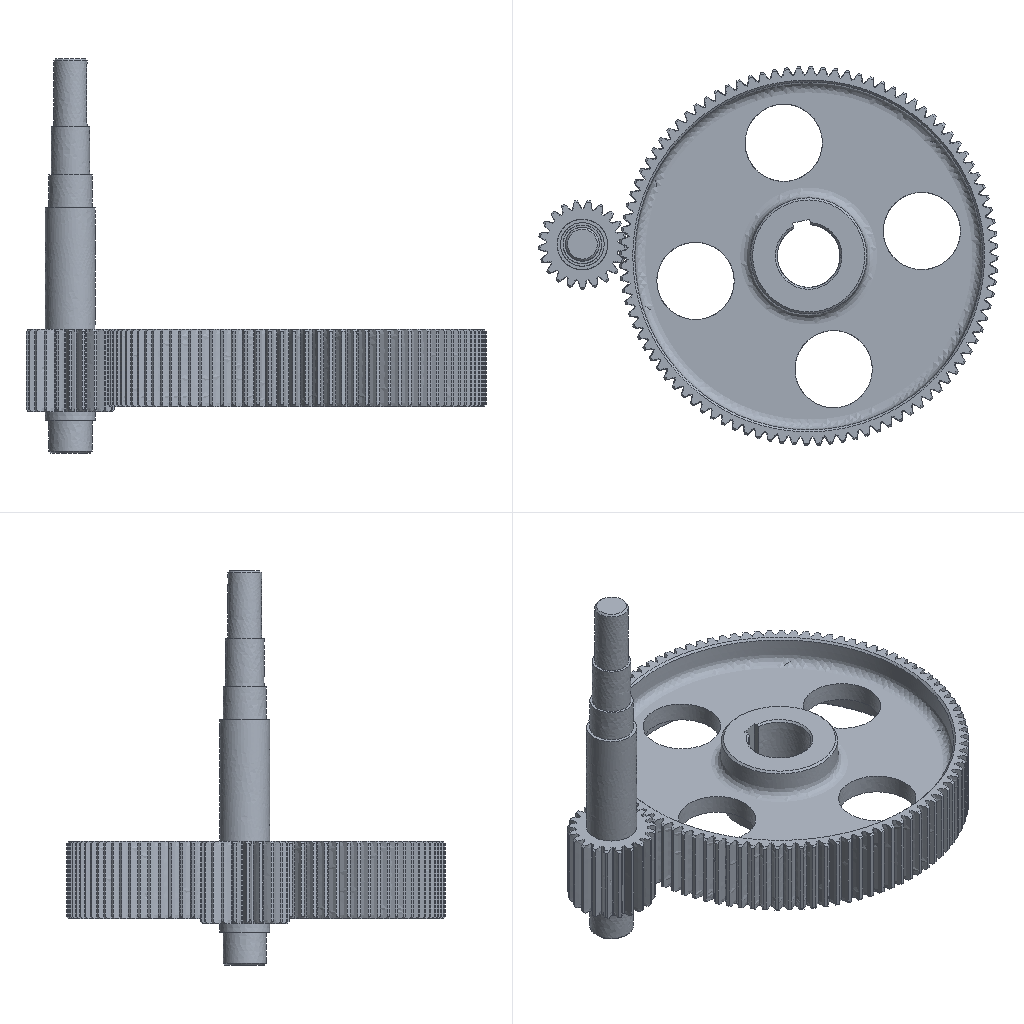Simulation study | ansys workbench
Ansys APDL input file, long lists of numbers shortened:
/batch
/config,noeldb,1     ! force off writing results to database
*get,_wallstrt,active,,time,wall
! ANSYS input file written by Workbench version 2022 R1
! File used for geometry attach:
/title,wbnew--__ (B5)
! ****** Begin Custom Load Command Snippet ******
/COM, ACT Extensions:
/COM,     LSDYNA, 2021.1
/COM,
! ****** End   Custom Load Command Snippet ******
*DIM,_wb_ProjectScratch_dir,string,248
_wb_ProjectScratch_dir(1) = ''
*DIM,_wb_SolverFiles_dir,string,248
_wb_SolverFiles_dir(1) = ''
*DIM,_wb_userfiles_dir,string,248
_wb_userfiles_dir(1) = ''
/com,--- Data in consistent NMM units. See Solving Units in the help system for more information.
/units,MPA
/nopr
/wb,file,start              !  signify a WB generated input file
/prep7
! Turn off shape checking because checks already performed inside WB mesher.
! See help system for more information.
SHPP,OFF,,NOWARN
/nolist
etcon,set             ! allow ANSYS to choose best KEYOP's for 180x elements, resets any applicable keyopt to MAPDL defaults
/com,*********** Nodes for the whole assembly ***********
nblock,3,,241700
(1i9,3e20.9e3)
        1    -2.217870232E+02     6.656718261E+00     2.175000000E+02
! (219727 more lines like these left out)
-1
/wb,elem,start            !  set before creation of elements
/com,*********** Elements for Body 1 "f7f8f6e2" ***********
et,1,187
eblock,19,solid,,94285
(19i9)
        1        1        1        1        0        0        0        0       10        0    28509    74937    77514    75585    76270   215855   218017   215849   215852
! (188569 more lines like these left out)
-1
/com,*********** Elements for Body 2 "ad8901f9f7f8f6e8f74" ***********
et,2,187
eblock,19,solid,,28508
(19i9)
        2        2        2        2        0        0        0        0       10        0        1     2002     2022     2023     8039    19195    19361    19196    19203
! (57015 more lines like these left out)
-1
/wb,elem,end               !  done creating elements
/com,*********** Send User Defined Coordinate System(s) ***********
csys,0
toffst,273.15,  ! Temperature offset from absolute zero
/com,*********** Set Reference Temperature ***********
tref,22.
/wb,mat,start              !  starting to send materials
/com,*********** Send Materials ***********
Temperature = 'TEMP' ! Temperature
MP,DENS,1,7.85e-09,	! tonne mm^-3
MP,ALPX,1,1.2e-05,	! C^-1
MP,C,1,434000000,	! mm^2 s^-2 C^-1
MP,KXX,1,60.5,	! tonne mm s^-3 C^-1
MP,RSVX,1,0.00017,	! ohm mm
MP,EX,1,200000,	! tonne s^-2 mm^-1
MP,NUXY,1,0.3,
MP,MURX,1,10000,
Temperature = 'TEMP' ! Temperature
MP,DENS,2,7.85e-09,	! tonne mm^-3
MP,ALPX,2,1.2e-05,	! C^-1
MP,C,2,434000000,	! mm^2 s^-2 C^-1
MP,KXX,2,60.5,	! tonne mm s^-3 C^-1
MP,RSVX,2,0.00017,	! ohm mm
MP,EX,2,200000,	! tonne s^-2 mm^-1
MP,NUXY,2,0.3,
MP,MURX,2,10000,
/wb,mat,end                !  done sending materials
!************************* Model Summary ********************
!f7f8f6e2,	结构钢,	matid,	1
!ad8901f9f7f8f6e8f74,	结构钢,	matid,	2
!************************* End Model Summary ********************
! get the diagonal of the bounding box. Needed later for other things
*get,_xmin,node,,mnloc,x
*get,_ymin,node,,mnloc,y
*get,_zmin,node,,mnloc,z
*get,_xmax,node,,mxloc,x
*get,_ymax,node,,mxloc,y
*get,_zmax,node,,mxloc,z
_ASMDIAG=(_xmax-_xmin)*(_xmax-_xmin)+(_ymax-_ymin)*(_ymax-_ymin)+(_zmax-_zmin)*(_zmax-_zmin)
_ASMDIAG=SQRT(_ASMDIAG)
/wb,contact,start          !  starting to send contact
/wb,contact,end            !  done creating contacts
/golist
/wb,load,start             !  starting to send loads
/com,********* Frictionless Supports X *********
CMBLOCK,_FRICSUX,NODE,     8519
(8i10)
       330       331       332       333       334       335       336       337
! (1064 more lines like these left out)
cmsel,s,_FRICSUX
d,all,ux,0
nsel,all
/com,********* Frictionless Supports Z *********
CMBLOCK,_FRICSUZ,NODE,     8519
(8i10)
       330       331       332       333       334       335       336       337
! (1064 more lines like these left out)
cmsel,s,_FRICSUZ
d,all,uz,0
nsel,all
/com,*********** Node Rotations ***********
nmod,330,,,,180.,0.,0.
nmod,331,,,,-171.22,0.,0.
nmod,332,,,,-162.439,0.,0.
nmod,333,,,,-153.659,0.,0.
! (8513 more lines like these left out)
/gst,on,on
fini
*get,_numnode,node,0,count
*get,_numelem,elem,0,count
*get, _MAXELEMNUM, elem, 0, NUM, MAX
*get, _MAXNODENUM, node, 0, NUM, MAX
*get, _MAXELEMTYPE, etyp, 0, NUM, MAX
*get, _MAXREALCONST, real, 0, NUM, MAX
/go
/wb,load,end               !  done creating loads
/com,--- Number of total nodes = %_numnode%
/com,--- Number of contact elements = 0
/com,--- Number of spring elements = 0
/com,--- Number of bearing elements = 0
/com,--- Number of solid elements = 122793
/com,--- Number of condensed parts = 0
/com,--- Number of total elements = %_numelem%
*get,_wallbsol,active,,time,wall
/solu
antype,2                   ! modal analysis
_thickRatio=  1     ! Ratio of thick parts in the model
modopt,lanb,10
outres,erase
outres,all,none
outres,nsol,all
outres,etmp,all
mxpand                    ! default expand in case of complex solution
dmpopt,esav,no
dmpopt,emat,no
dmpopt,full,no
! *********** WB SOLVE COMMAND ***********
! check interactive state
*get,ANSINTER_,active,,int
*if,ANSINTER_,ne,0,then
/eof
*endif
solve
/com *************** Write FE CONNECTORS *********
CEWRITE,file,ce,,INTE
*get,_nmodalsolproc,active,0,numcpu
fini
/nopr
*get,_numnode,node,0,count
*get,_numelem,elem,0,count
*get, _MAXELEMNUM, elem, 0, NUM, MAX
*get, _MAXNODENUM, node, 0, NUM, MAX,,,INTERNAL
*get, _MAXELEMTYPE, etyp, 0, NUM, MAX
*get, _MAXREALCONST, real, 0, NUM, MAX
/gopr
*get,_wallasol,active,,time,wall
/post1
/nopr
*dim,_direction,CHAR,6,1
_direction(1) = 'X'
_direction(2) = 'Y'
_direction(3) = 'Z'
_direction(4) = 'ROTX'
_direction(5) = 'ROTY'
_direction(6) = 'ROTZ'
*get,_lastLS,active,0,set,LSTP
*get,_beginset,active,0,set,nset,first,_lastLS
*get,_endset,active,0,set,nset,last,_lastLS
_nummodes = 0
*if,_endset,gt,0,then
_nummodes = _endset - _beginset + 1
*endif
*do,i_mode,1,_nummodes
   *do,j_component,1,6
			*get,PFACT_%i_mode%_%j_component%,MODE,%i_mode%,PFACT,,DIREC,_direction(%j_component%)
   *enddo
*enddo
*dim,_tmdirection,CHAR,6,1
_tmdirection(1) = 'X'
_tmdirection(2) = 'Y'
_tmdirection(3) = 'Z'
_tmdirection(4) = 'X'
_tmdirection(5) = 'Y'
_tmdirection(6) = 'Z'
*do,j_component,1,6
    *if,j_component,gt,3,then
        *get,TOTALMASS_%j_component%,ELEM,0,IOR,_tmdirection(%j_component%)
    *else
        *get,TOTALMASS_%j_component%,ELEM,0,MTOT,_tmdirection(%j_component%)
    *endif
*enddo
/gopr
xmlo,ENCODING,ISO-8859-1
xmlo,parm
/xml,parm,xml
fini
/gopr
*get,_walldone,active,,time,wall
_preptime=(_wallbsol-_wallstrt)*3600
_solvtime=(_wallasol-_wallbsol)*3600
_posttime=(_walldone-_wallasol)*3600
_totaltim=(_walldone-_wallstrt)*3600
*get,_dlbratio,active,0,solu,dlbr
*get,_combtime,active,0,solu,comb
*get,_ssmode,active,0,solu,ssmm
*get,_ndofs,active,0,solu,ndof
/fclean				!clean distributed files
/com,--- Total number of nodes = %_numnode%
/com,--- Total number of elements = %_numelem%
/com,--- Element load balance ratio = %_dlbratio%
/com,--- Time to combine distributed files = %_combtime%
/com,--- Sparse memory mode = %_ssmode%
/com,--- Number of DOF = %_ndofs%
/wb,file,end               ! done with WB generated input